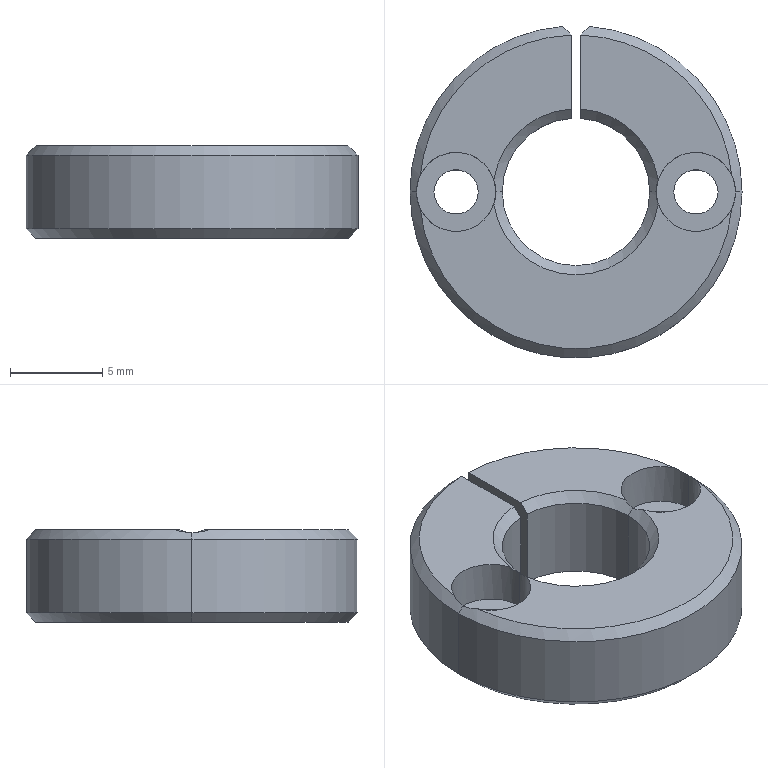Part | STEP file | 08 displacement fixing | 1 solid | 33 faces | box 18 x 17.971 x 5 mm | volume 899.318 mm3 | cylinder 14 | plane 10 | cone 9 | commonest cylinder face diameters 2.4 x4 4.3 x4 8 x3 18 x3